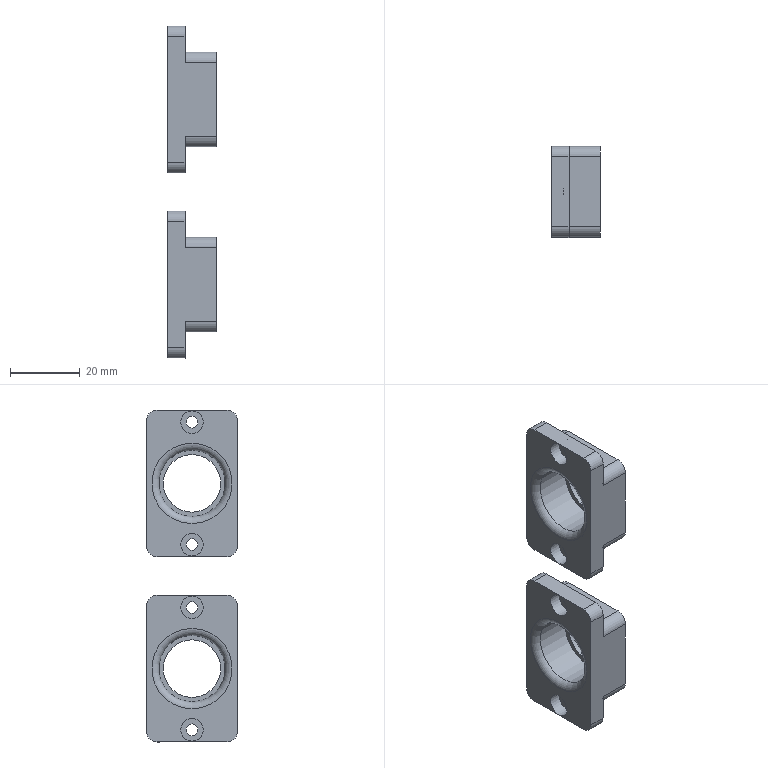Part | 2 solids | 56 faces | box 14 x 26 x 95 mm | volume 15063 mm3 | cylinder 28 | plane 26 | torus 2 | commonest cylinder face diameters 6 x16 3.4 x4 6.5 x4 16.5 x2 19 x2